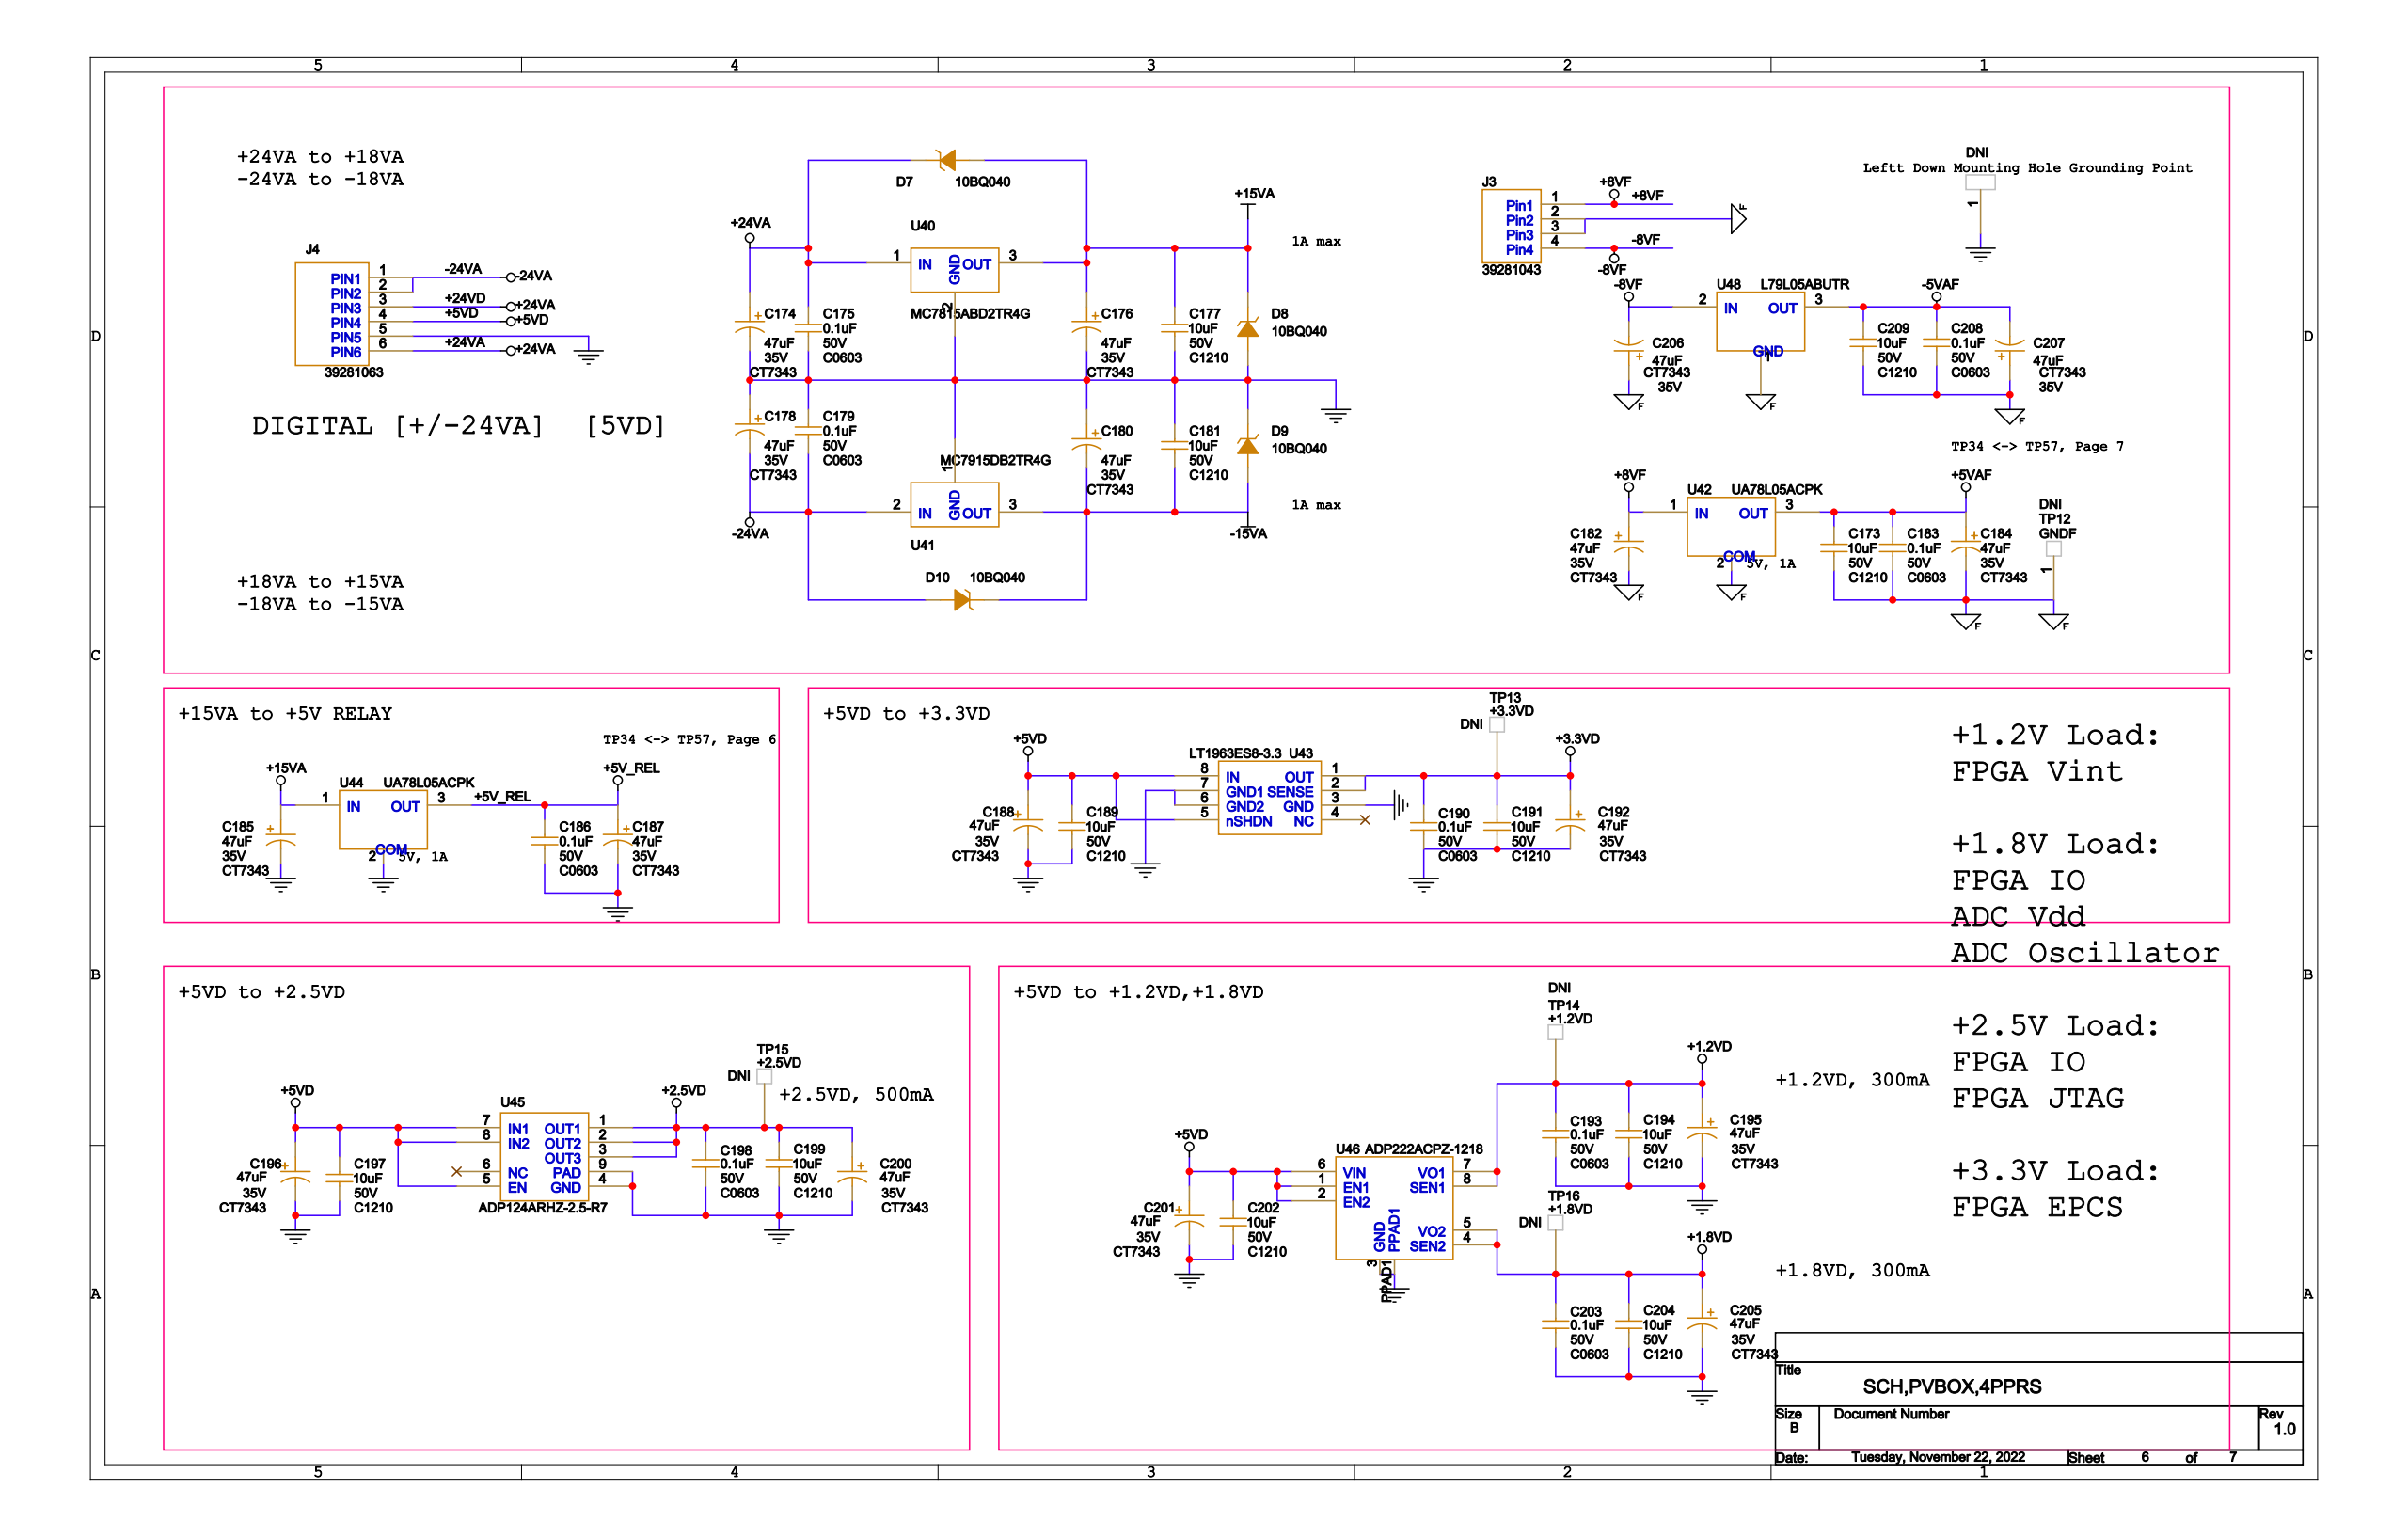Circuit board | Cadence Allegro | 405 parts | 254 nets | one sheet of the schematic
Parts on this sheet (reference | value | footprint):
C173 | C1210
C174 | CT7343
C175 | C0603
C176 | CT7343
C177 | C1210
C178 | CT7343
C179 | C0603
C180 | CT7343
C181 | C1210
C182 | CT7343
C183 | C0603
C184 | CT7343
C185 | CT7343
C186 | C0603
C187 | CT7343
C189 | C1210
C190 | C0603
C191 | C1210
C192 | CT7343
C193 | C0603
C194 | C1210
C195 | CT7343
C197 | C1210
C198 | C0603
C199 | C1210
C200 | CT7343
C202 | C1210
C203 | C0603
C204 | C1210
C205 | CT7343
C207 | CT7343
C208 | C0603
C209 | C1210
D7 | DO-214AA
D8 | DO-214AA
D9 | DO-214AA
D10 | DO-214AA
J3 | 39281043
J4 | 39281063
TP12 | TP_0M8X1M15
TP13 | TP_0M8X1M15
TP14 | TP_0M8X1M15
TP15 | TP_0M8X1M15
TP16 | TP_0M8X1M15
U40 | TO-263-2
U41 | TO-263-2
U42 | UA78L05ACPK_SOT_3
U43 | SOIC_8_4MX5MX1M75_1M27
U44 | UA78L05ACPK_SOT_3
U45 | MINI_SO_EP_8
U46 | DFN_9_2M1X2M1X0M6_0M5
U48 | L79L05ABUTR
Nets of these parts (net: part-pin ...):
GND: C174-2 C175-2 C176-2 C177-2 C178-1 C179-1 C180-1 C181-1 C185-2 C186-2 C187-2 C189-2 C190-2 C191-2 C192-2 C193-2 C194-2 C195-2 C197-2 C198-2 C199-2 C200-2 C202-2 C203-2 C204-2 C205-2 D8-1 D9-2 J4-5 U40-2 U41-1 U43-3 U43-6 U43-7 U44-2 U45-4 U45-9 U46-3 U46-PPAD1
+2.5VD: C198-1 C199-1 C200-1 TP15-1 U45-1 U45-2 U45-3
+3.3VD: C190-1 C191-1 C192-1 TP13-1 U43-1 U43-2
+1.8VD: C203-1 C204-1 C205-1 TP16-1 U46-4 U46-5
+1.2VD: C193-1 C194-1 C195-1 TP14-1 U46-7 U46-8
+24VA: C174-1 C175-1 D7-2 J4-3 J4-6 U40-1
-24VA: C178-2 C179-2 D10-1 J4-1 J4-2 U41-2
+5VAF: C173-1 C183-1 C184-1 U42-3
GNDF: C173-2 C182-2 C183-2 C184-2 C207-1 C208-2 C209-2 J3-2 J3-3 TP12-1 U42-2 U48-1
+5V_REL: C186-1 C187-1 U44-3
+15VA: C176-1 C177-1 C185-1 D7-1 D8-2 U40-3 U44-1
-5VAF: C207-2 C208-1 C209-1 U48-3
-15VA: C180-2 C181-2 D9-1 D10-2 U41-3
+5VD: C189-1 C197-1 C202-1 J4-4 U43-5 U43-8 U45-5 U45-7 U45-8 U46-1 U46-2 U46-6
+8VF: C182-1 J3-1 U42-1
-8VF: J3-4 U48-2